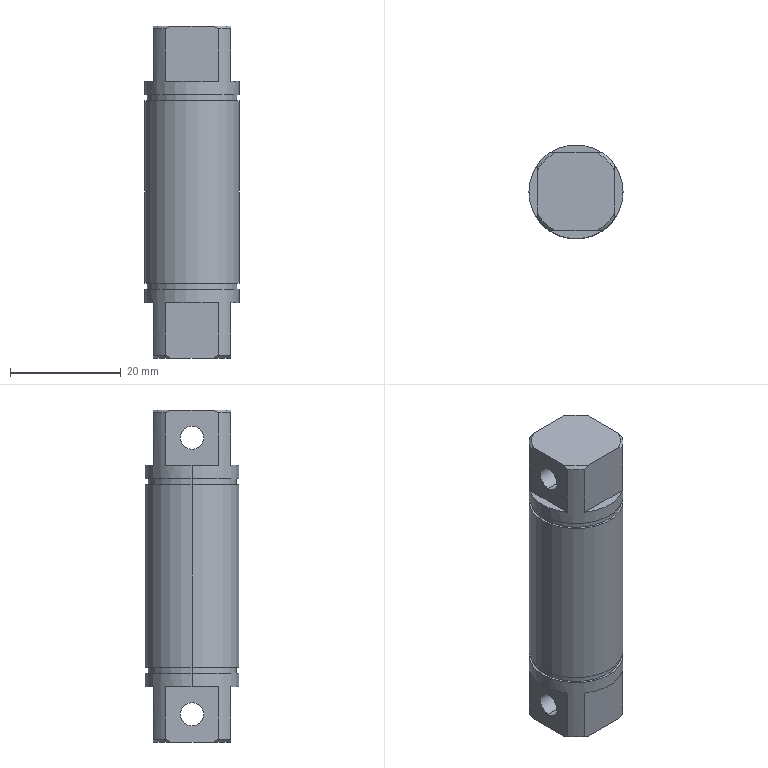Part | SolidWorks | features MirrorPattern 2, Chamfer 1, Extrusion 1, HoleWzd 1, ICE 1, RevCut 1 | 1 solid | 44 faces | box 17 x 17 x 60 mm | volume 12395 mm3 | plane 22 | cylinder 14 | cone 8 | commonest cylinder face diameters 17 x6 4.2 x4 16.2 x4
STEP:
#1=CARTESIAN_POINT('',(8.5,0.,20.));
#2=VERTEX_POINT('',#1);
#3=CARTESIAN_POINT('',(7.,4.822,20.));
#4=VERTEX_POINT('',#3);
#5=CARTESIAN_POINT('',(0.,0.,20.));
#6=DIRECTION('',(0.,0.,1.));
#7=DIRECTION('',(1.,0.,0.));
#8=AXIS2_PLACEMENT_3D('',#5,#6,#7);
#9=CIRCLE('',#8,8.5);
#10=EDGE_CURVE('',#2,#4,#9,.T.);
#11=ORIENTED_EDGE('',*,*,#10,.F.);
#12=CARTESIAN_POINT('',(8.5,0.,17.6));
#13=VERTEX_POINT('',#12);
#14=CARTESIAN_POINT('',(8.5,0.,30.));
#15=DIRECTION('',(0.,0.,-1.));
#16=VECTOR('',#15,1000.);
#17=LINE('',#14,#16);
#18=EDGE_CURVE('',#2,#13,#17,.T.);
#19=ORIENTED_EDGE('',*,*,#18,.T.);
#20=CARTESIAN_POINT('',(-8.5,0.,17.6));
#21=VERTEX_POINT('',#20);
#22=CARTESIAN_POINT('',(0.,0.,17.6));
#23=DIRECTION('',(0.,0.,-1.));
#24=DIRECTION('',(-1.,0.,0.));
#25=AXIS2_PLACEMENT_3D('',#22,#23,#24);
#26=CIRCLE('',#25,8.5);
#27=EDGE_CURVE('',#21,#13,#26,.T.);
#28=ORIENTED_EDGE('',*,*,#27,.F.);
#29=CARTESIAN_POINT('',(-8.5,0.,20.));
#30=VERTEX_POINT('',#29);
#31=CARTESIAN_POINT('',(-8.5,0.,30.));
#32=DIRECTION('',(0.,0.,-1.));
#33=VECTOR('',#32,1000.);
#34=LINE('',#31,#33);
#35=EDGE_CURVE('',#30,#21,#34,.T.);
#36=ORIENTED_EDGE('',*,*,#35,.F.);
#37=CARTESIAN_POINT('',(-7.,4.822,20.));
#38=VERTEX_POINT('',#37);
#39=CARTESIAN_POINT('',(0.,0.,20.));
#40=DIRECTION('',(0.,0.,1.));
#41=DIRECTION('',(1.,0.,0.));
#42=AXIS2_PLACEMENT_3D('',#39,#40,#41);
#43=CIRCLE('',#42,8.5);
#44=EDGE_CURVE('',#38,#30,#43,.T.);
#45=ORIENTED_EDGE('',*,*,#44,.F.);
#46=CARTESIAN_POINT('',(-7.,4.822,29.5));
#47=VERTEX_POINT('',#46);
#48=CARTESIAN_POINT('',(-7.,4.822,30.));
#49=DIRECTION('',(0.,0.,-1.));
#50=VECTOR('',#49,1000.);
#51=LINE('',#48,#50);
#52=EDGE_CURVE('',#47,#38,#51,.T.);
#53=ORIENTED_EDGE('',*,*,#52,.F.);
#54=CARTESIAN_POINT('',(-4.822,7.,29.5));
#55=VERTEX_POINT('',#54);
#56=CARTESIAN_POINT('',(0.,0.,29.5));
#57=DIRECTION('',(0.,0.,-1.));
#58=DIRECTION('',(1.,0.,0.));
#59=AXIS2_PLACEMENT_3D('',#56,#57,#58);
#60=CIRCLE('',#59,8.5);
#61=EDGE_CURVE('',#47,#55,#60,.T.);
#62=ORIENTED_EDGE('',*,*,#61,.T.);
#63=CARTESIAN_POINT('',(-4.822,7.,20.));
#64=VERTEX_POINT('',#63);
#65=CARTESIAN_POINT('',(-4.822,7.,30.));
#66=DIRECTION('',(0.,0.,1.));
#67=VECTOR('',#66,1000.);
#68=LINE('',#65,#67);
#69=EDGE_CURVE('',#64,#55,#68,.T.);
#70=ORIENTED_EDGE('',*,*,#69,.F.);
#71=CARTESIAN_POINT('',(4.822,7.,20.));
#72=VERTEX_POINT('',#71);
#73=CARTESIAN_POINT('',(0.,0.,20.));
#74=DIRECTION('',(0.,0.,1.));
#75=DIRECTION('',(1.,0.,0.));
#76=AXIS2_PLACEMENT_3D('',#73,#74,#75);
#77=CIRCLE('',#76,8.5);
#78=EDGE_CURVE('',#72,#64,#77,.T.);
#79=ORIENTED_EDGE('',*,*,#78,.F.);
#80=CARTESIAN_POINT('',(4.822,7.,29.5));
#81=VERTEX_POINT('',#80);
#82=CARTESIAN_POINT('',(4.822,7.,30.));
#83=DIRECTION('',(0.,0.,-1.));
#84=VECTOR('',#83,1000.);
#85=LINE('',#82,#84);
#86=EDGE_CURVE('',#81,#72,#85,.T.);
#87=ORIENTED_EDGE('',*,*,#86,.F.);
#88=CARTESIAN_POINT('',(7.,4.822,29.5));
#89=VERTEX_POINT('',#88);
#90=CARTESIAN_POINT('',(0.,0.,29.5));
#91=DIRECTION('',(0.,0.,-1.));
#92=DIRECTION('',(1.,0.,0.));
#93=AXIS2_PLACEMENT_3D('',#90,#91,#92);
#94=CIRCLE('',#93,8.5);
#95=EDGE_CURVE('',#81,#89,#94,.T.);
#96=ORIENTED_EDGE('',*,*,#95,.T.);
#97=CARTESIAN_POINT('',(7.,4.822,30.));
#98=DIRECTION('',(0.,0.,1.));
#99=VECTOR('',#98,1000.);
#100=LINE('',#97,#99);
#101=EDGE_CURVE('',#4,#89,#100,.T.);
#102=ORIENTED_EDGE('',*,*,#101,.F.);
#103=EDGE_LOOP('',(#11,#19,#28,#36,#45,#53,#62,#70,#79,#87,#96,#102));
#104=FACE_OUTER_BOUND('',#103,.T.);
#105=CARTESIAN_POINT('',(0.,0.,30.));
#106=DIRECTION('',(0.,0.,-1.));
#107=DIRECTION('',(-1.,0.,0.));
#108=AXIS2_PLACEMENT_3D('',#105,#106,#107);
#109=CYLINDRICAL_SURFACE('',#108,8.5);
#110=ADVANCED_FACE('',(#104),#109,.T.);
#111=CARTESIAN_POINT('',(-7.,0.,22.9));
#112=VERTEX_POINT('',#111);
#113=CARTESIAN_POINT('',(-7.,0.,27.1));
#114=VERTEX_POINT('',#113);
#115=CARTESIAN_POINT('',(-7.,0.,25.));
#116=DIRECTION('',(-1.,0.,0.));
#117=DIRECTION('',(0.,-1.,0.));
#118=AXIS2_PLACEMENT_3D('',#115,#116,#117);
#119=CIRCLE('',#118,2.1);
#120=EDGE_CURVE('',#112,#114,#119,.T.);
#121=ORIENTED_EDGE('',*,*,#120,.T.);
#122=CARTESIAN_POINT('',(7.,0.,27.1));
#123=VERTEX_POINT('',#122);
#124=CARTESIAN_POINT('',(7.,0.,27.1));
#125=DIRECTION('',(1.,0.,0.));
#126=VECTOR('',#125,1000.);
#127=LINE('',#124,#126);
#128=EDGE_CURVE('',#114,#123,#127,.T.);
#129=ORIENTED_EDGE('',*,*,#128,.T.);
#130=CARTESIAN_POINT('',(7.,0.,22.9));
#131=VERTEX_POINT('',#130);
#132=CARTESIAN_POINT('',(7.,0.,25.));
#133=DIRECTION('',(1.,0.,0.));
#134=DIRECTION('',(0.,0.,-1.));
#135=AXIS2_PLACEMENT_3D('',#132,#133,#134);
#136=CIRCLE('',#135,2.1);
#137=EDGE_CURVE('',#123,#131,#136,.T.);
#138=ORIENTED_EDGE('',*,*,#137,.T.);
#139=CARTESIAN_POINT('',(7.,0.,22.9));
#140=DIRECTION('',(1.,0.,0.));
#141=VECTOR('',#140,1000.);
#142=LINE('',#139,#141);
#143=EDGE_CURVE('',#112,#131,#142,.T.);
#144=ORIENTED_EDGE('',*,*,#143,.F.);
#145=EDGE_LOOP('',(#121,#129,#138,#144));
#146=FACE_OUTER_BOUND('',#145,.T.);
#147=CARTESIAN_POINT('',(7.,0.,25.));
#148=DIRECTION('',(1.,0.,0.));
#149=DIRECTION('',(0.,0.,-1.));
#150=AXIS2_PLACEMENT_3D('',#147,#148,#149);
#151=CYLINDRICAL_SURFACE('',#150,2.1);
#152=ADVANCED_FACE('',(#146),#151,.F.);
#153=CARTESIAN_POINT('',(8.1,0.,16.5));
#154=VERTEX_POINT('',#153);
#155=CARTESIAN_POINT('',(-8.1,0.,16.5));
#156=VERTEX_POINT('',#155);
#157=CARTESIAN_POINT('',(0.,0.,16.5));
#158=DIRECTION('',(0.,0.,-1.));
#159=DIRECTION('',(-1.,0.,0.));
#160=AXIS2_PLACEMENT_3D('',#157,#158,#159);
#161=CIRCLE('',#160,8.1);
#162=EDGE_CURVE('',#154,#156,#161,.T.);
#163=ORIENTED_EDGE('',*,*,#162,.F.);
#164=CARTESIAN_POINT('',(8.1,0.,17.6));
#165=VERTEX_POINT('',#164);
#166=CARTESIAN_POINT('',(8.1,0.,14.765));
#167=DIRECTION('',(0.,0.,1.));
#168=VECTOR('',#167,1000.);
#169=LINE('',#166,#168);
#170=EDGE_CURVE('',#154,#165,#169,.T.);
#171=ORIENTED_EDGE('',*,*,#170,.T.);
#172=CARTESIAN_POINT('',(-8.1,0.,17.6));
#173=VERTEX_POINT('',#172);
#174=CARTESIAN_POINT('',(0.,0.,17.6));
#175=DIRECTION('',(0.,0.,-1.));
#176=DIRECTION('',(-1.,0.,0.));
#177=AXIS2_PLACEMENT_3D('',#174,#175,#176);
#178=CIRCLE('',#177,8.1);
#179=EDGE_CURVE('',#165,#173,#178,.T.);
#180=ORIENTED_EDGE('',*,*,#179,.T.);
#181=CARTESIAN_POINT('',(-8.1,0.,14.765));
#182=DIRECTION('',(0.,0.,1.));
#183=VECTOR('',#182,1000.);
#184=LINE('',#181,#183);
#185=EDGE_CURVE('',#156,#173,#184,.T.);
#186=ORIENTED_EDGE('',*,*,#185,.F.);
#187=EDGE_LOOP('',(#163,#171,#180,#186));
#188=FACE_OUTER_BOUND('',#187,.T.);
#189=CARTESIAN_POINT('',(0.,0.,14.765));
#190=DIRECTION('',(0.,0.,1.));
#191=DIRECTION('',(-1.,0.,0.));
#192=AXIS2_PLACEMENT_3D('',#189,#190,#191);
#193=CYLINDRICAL_SURFACE('',#192,8.1);
#194=ADVANCED_FACE('',(#188),#193,.T.);
#195=CARTESIAN_POINT('',(-8.5,0.,-17.6));
#196=VERTEX_POINT('',#195);
#197=CARTESIAN_POINT('',(8.5,0.,-17.6));
#198=VERTEX_POINT('',#197);
#199=CARTESIAN_POINT('',(0.,0.,-17.6));
#200=DIRECTION('',(0.,0.,-1.));
#201=DIRECTION('',(-1.,0.,0.));
#202=AXIS2_PLACEMENT_3D('',#199,#200,#201);
#203=CIRCLE('',#202,8.5);
#204=EDGE_CURVE('',#196,#198,#203,.T.);
#205=ORIENTED_EDGE('',*,*,#204,.T.);
#206=CARTESIAN_POINT('',(8.5,0.,-20.));
#207=VERTEX_POINT('',#206);
#208=CARTESIAN_POINT('',(8.5,0.,30.));
#209=DIRECTION('',(0.,0.,-1.));
#210=VECTOR('',#209,1000.);
#211=LINE('',#208,#210);
#212=EDGE_CURVE('',#198,#207,#211,.T.);
#213=ORIENTED_EDGE('',*,*,#212,.T.);
#214=CARTESIAN_POINT('',(7.,4.822,-20.));
#215=VERTEX_POINT('',#214);
#216=CARTESIAN_POINT('',(0.,0.,-20.));
#217=DIRECTION('',(0.,0.,-1.));
#218=DIRECTION('',(-1.,0.,0.));
#219=AXIS2_PLACEMENT_3D('',#216,#217,#218);
#220=CIRCLE('',#219,8.5);
#221=EDGE_CURVE('',#215,#207,#220,.T.);
#222=ORIENTED_EDGE('',*,*,#221,.F.);
#223=CARTESIAN_POINT('',(7.,4.822,-29.5));
#224=VERTEX_POINT('',#223);
#225=CARTESIAN_POINT('',(7.,4.822,30.));
#226=DIRECTION('',(0.,0.,-1.));
#227=VECTOR('',#226,1000.);
#228=LINE('',#225,#227);
#229=EDGE_CURVE('',#215,#224,#228,.T.);
#230=ORIENTED_EDGE('',*,*,#229,.T.);
#231=CARTESIAN_POINT('',(4.822,7.,-29.5));
#232=VERTEX_POINT('',#231);
#233=CARTESIAN_POINT('',(0.,0.,-29.5));
#234=DIRECTION('',(0.,0.,1.));
#235=DIRECTION('',(1.,0.,0.));
#236=AXIS2_PLACEMENT_3D('',#233,#234,#235);
#237=CIRCLE('',#236,8.5);
#238=EDGE_CURVE('',#224,#232,#237,.T.);
#239=ORIENTED_EDGE('',*,*,#238,.T.);
#240=CARTESIAN_POINT('',(4.822,7.,-20.));
#241=VERTEX_POINT('',#240);
#242=CARTESIAN_POINT('',(4.822,7.,30.));
#243=DIRECTION('',(0.,0.,1.));
#244=VECTOR('',#243,1000.);
#245=LINE('',#242,#244);
#246=EDGE_CURVE('',#232,#241,#245,.T.);
#247=ORIENTED_EDGE('',*,*,#246,.T.);
#248=CARTESIAN_POINT('',(-4.822,7.,-20.));
#249=VERTEX_POINT('',#248);
#250=CARTESIAN_POINT('',(0.,0.,-20.));
#251=DIRECTION('',(0.,0.,-1.));
#252=DIRECTION('',(-1.,0.,0.));
#253=AXIS2_PLACEMENT_3D('',#250,#251,#252);
#254=CIRCLE('',#253,8.5);
#255=EDGE_CURVE('',#249,#241,#254,.T.);
#256=ORIENTED_EDGE('',*,*,#255,.F.);
#257=CARTESIAN_POINT('',(-4.822,7.,-29.5));
#258=VERTEX_POINT('',#257);
#259=CARTESIAN_POINT('',(-4.822,7.,30.));
#260=DIRECTION('',(0.,0.,-1.));
#261=VECTOR('',#260,1000.);
#262=LINE('',#259,#261);
#263=EDGE_CURVE('',#249,#258,#262,.T.);
#264=ORIENTED_EDGE('',*,*,#263,.T.);
#265=CARTESIAN_POINT('',(-7.,4.822,-29.5));
#266=VERTEX_POINT('',#265);
#267=CARTESIAN_POINT('',(0.,0.,-29.5));
#268=DIRECTION('',(0.,0.,1.));
#269=DIRECTION('',(1.,0.,0.));
#270=AXIS2_PLACEMENT_3D('',#267,#268,#269);
#271=CIRCLE('',#270,8.5);
#272=EDGE_CURVE('',#258,#266,#271,.T.);
#273=ORIENTED_EDGE('',*,*,#272,.T.);
#274=CARTESIAN_POINT('',(-7.,4.822,-20.));
#275=VERTEX_POINT('',#274);
#276=CARTESIAN_POINT('',(-7.,4.822,30.));
#277=DIRECTION('',(0.,0.,1.));
#278=VECTOR('',#277,1000.);
#279=LINE('',#276,#278);
#280=EDGE_CURVE('',#266,#275,#279,.T.);
#281=ORIENTED_EDGE('',*,*,#280,.T.);
#282=CARTESIAN_POINT('',(-8.5,0.,-20.));
#283=VERTEX_POINT('',#282);
#284=CARTESIAN_POINT('',(0.,0.,-20.));
#285=DIRECTION('',(0.,0.,-1.));
#286=DIRECTION('',(-1.,0.,0.));
#287=AXIS2_PLACEMENT_3D('',#284,#285,#286);
#288=CIRCLE('',#287,8.5);
#289=EDGE_CURVE('',#283,#275,#288,.T.);
#290=ORIENTED_EDGE('',*,*,#289,.F.);
#291=CARTESIAN_POINT('',(-8.5,0.,30.));
#292=DIRECTION('',(0.,0.,-1.));
#293=VECTOR('',#292,1000.);
#294=LINE('',#291,#293);
#295=EDGE_CURVE('',#196,#283,#294,.T.);
#296=ORIENTED_EDGE('',*,*,#295,.F.);
#297=EDGE_LOOP('',(#205,#213,#222,#230,#239,#247,#256,#264,#273,#281,#290,#296));
#298=FACE_OUTER_BOUND('',#297,.T.);
#299=CARTESIAN_POINT('',(0.,0.,30.));
#300=DIRECTION('',(0.,0.,-1.));
#301=DIRECTION('',(-1.,0.,0.));
#302=AXIS2_PLACEMENT_3D('',#299,#300,#301);
#303=CYLINDRICAL_SURFACE('',#302,8.5);
#304=ADVANCED_FACE('',(#298),#303,.T.);
#305=CARTESIAN_POINT('',(-7.,0.,-22.9));
#306=VERTEX_POINT('',#305);
#307=CARTESIAN_POINT('',(-7.,0.,-27.1));
#308=VERTEX_POINT('',#307);
#309=CARTESIAN_POINT('',(-7.,0.,-25.));
#310=DIRECTION('',(1.,0.,0.));
#311=DIRECTION('',(0.,1.,0.));
#312=AXIS2_PLACEMENT_3D('',#309,#310,#311);
#313=CIRCLE('',#312,2.1);
#314=EDGE_CURVE('',#306,#308,#313,.T.);
#315=ORIENTED_EDGE('',*,*,#314,.F.);
#316=CARTESIAN_POINT('',(7.,0.,-22.9));
#317=VERTEX_POINT('',#316);
#318=CARTESIAN_POINT('',(7.,0.,-22.9));
#319=DIRECTION('',(1.,0.,0.));
#320=VECTOR('',#319,1000.);
#321=LINE('',#318,#320);
#322=EDGE_CURVE('',#306,#317,#321,.T.);
#323=ORIENTED_EDGE('',*,*,#322,.T.);
#324=CARTESIAN_POINT('',(7.,0.,-27.1));
#325=VERTEX_POINT('',#324);
#326=CARTESIAN_POINT('',(7.,0.,-25.));
#327=DIRECTION('',(1.,0.,0.));
#328=DIRECTION('',(0.,0.,-1.));
#329=AXIS2_PLACEMENT_3D('',#326,#327,#328);
#330=CIRCLE('',#329,2.1);
#331=EDGE_CURVE('',#317,#325,#330,.T.);
#332=ORIENTED_EDGE('',*,*,#331,.T.);
#333=CARTESIAN_POINT('',(7.,0.,-27.1));
#334=DIRECTION('',(1.,0.,0.));
#335=VECTOR('',#334,1000.);
#336=LINE('',#333,#335);
#337=EDGE_CURVE('',#308,#325,#336,.T.);
#338=ORIENTED_EDGE('',*,*,#337,.F.);
#339=EDGE_LOOP('',(#315,#323,#332,#338));
#340=FACE_OUTER_BOUND('',#339,.T.);
#341=CARTESIAN_POINT('',(7.,0.,-25.));
#342=DIRECTION('',(1.,0.,0.));
#343=DIRECTION('',(0.,0.,-1.));
#344=AXIS2_PLACEMENT_3D('',#341,#342,#343);
#345=CYLINDRICAL_SURFACE('',#344,2.1);
#346=ADVANCED_FACE('',(#340),#345,.F.);
#347=CARTESIAN_POINT('',(-8.1,0.,-16.5));
#348=VERTEX_POINT('',#347);
#349=CARTESIAN_POINT('',(8.1,0.,-16.5));
#350=VERTEX_POINT('',#349);
#351=CARTESIAN_POINT('',(0.,0.,-16.5));
#352=DIRECTION('',(0.,0.,-1.));
#353=DIRECTION('',(-1.,0.,0.));
#354=AXIS2_PLACEMENT_3D('',#351,#352,#353);
#355=CIRCLE('',#354,8.1);
#356=EDGE_CURVE('',#348,#350,#355,.T.);
#357=ORIENTED_EDGE('',*,*,#356,.T.);
#358=CARTESIAN_POINT('',(8.1,0.,-17.6));
#359=VERTEX_POINT('',#358);
#360=CARTESIAN_POINT('',(8.1,0.,-14.765));
#361=DIRECTION('',(0.,0.,-1.));
#362=VECTOR('',#361,1000.);
#363=LINE('',#360,#362);
#364=EDGE_CURVE('',#350,#359,#363,.T.);
#365=ORIENTED_EDGE('',*,*,#364,.T.);
#366=CARTESIAN_POINT('',(-8.1,0.,-17.6));
#367=VERTEX_POINT('',#366);
#368=CARTESIAN_POINT('',(0.,0.,-17.6));
#369=DIRECTION('',(0.,0.,-1.));
#370=DIRECTION('',(-1.,0.,0.));
#371=AXIS2_PLACEMENT_3D('',#368,#369,#370);
#372=CIRCLE('',#371,8.1);
#373=EDGE_CURVE('',#367,#359,#372,.T.);
#374=ORIENTED_EDGE('',*,*,#373,.F.);
#375=CARTESIAN_POINT('',(-8.1,0.,-14.765));
#376=DIRECTION('',(0.,0.,-1.));
#377=VECTOR('',#376,1000.);
#378=LINE('',#375,#377);
#379=EDGE_CURVE('',#348,#367,#378,.T.);
#380=ORIENTED_EDGE('',*,*,#379,.F.);
#381=EDGE_LOOP('',(#357,#365,#374,#380));
#382=FACE_OUTER_BOUND('',#381,.T.);
#383=CARTESIAN_POINT('',(0.,0.,-14.765));
#384=DIRECTION('',(0.,0.,-1.));
#385=DIRECTION('',(-1.,0.,0.));
#386=AXIS2_PLACEMENT_3D('',#383,#384,#385);
#387=CYLINDRICAL_SURFACE('',#386,8.1);
#388=ADVANCED_FACE('',(#382),#387,.T.);
#389=CARTESIAN_POINT('',(-8.5,0.,16.5));
#390=VERTEX_POINT('',#389);
#391=CARTESIAN_POINT('',(8.5,0.,16.5));
#392=VERTEX_POINT('',#391);
#393=CARTESIAN_POINT('',(0.,0.,16.5));
#394=DIRECTION('',(0.,0.,-1.));
#395=DIRECTION('',(-1.,0.,0.));
#396=AXIS2_PLACEMENT_3D('',#393,#394,#395);
#397=CIRCLE('',#396,8.5);
#398=EDGE_CURVE('',#390,#392,#397,.T.);
#399=ORIENTED_EDGE('',*,*,#398,.T.);
#400=CARTESIAN_POINT('',(8.5,0.,-16.5));
#401=VERTEX_POINT('',#400);
#402=CARTESIAN_POINT('',(8.5,0.,30.));
#403=DIRECTION('',(0.,0.,-1.));
#404=VECTOR('',#403,1000.);
#405=LINE('',#402,#404);
#406=EDGE_CURVE('',#392,#401,#405,.T.);
#407=ORIENTED_EDGE('',*,*,#406,.T.);
#408=CARTESIAN_POINT('',(-8.5,0.,-16.5));
#409=VERTEX_POINT('',#408);
#410=CARTESIAN_POINT('',(0.,0.,-16.5));
#411=DIRECTION('',(0.,0.,-1.));
#412=DIRECTION('',(-1.,0.,0.));
#413=AXIS2_PLACEMENT_3D('',#410,#411,#412);
#414=CIRCLE('',#413,8.5);
#415=EDGE_CURVE('',#409,#401,#414,.T.);
#416=ORIENTED_EDGE('',*,*,#415,.F.);
#417=CARTESIAN_POINT('',(-8.5,0.,30.));
#418=DIRECTION('',(0.,0.,-1.));
#419=VECTOR('',#418,1000.);
#420=LINE('',#417,#419);
#421=EDGE_CURVE('',#390,#409,#420,.T.);
#422=ORIENTED_EDGE('',*,*,#421,.F.);
#423=EDGE_LOOP('',(#399,#407,#416,#422));
#424=FACE_OUTER_BOUND('',#423,.T.);
#425=CARTESIAN_POINT('',(0.,0.,30.));
#426=DIRECTION('',(0.,0.,-1.));
#427=DIRECTION('',(-1.,0.,0.));
#428=AXIS2_PLACEMENT_3D('',#425,#426,#427);
#429=CYLINDRICAL_SURFACE('',#428,8.5);
#430=ADVANCED_FACE('',(#424),#429,.T.);
#431=ORIENTED_EDGE('',*,*,#406,.F.);
#432=CARTESIAN_POINT('',(0.,0.,16.5));
#433=DIRECTION('',(0.,0.,-1.));
#434=DIRECTION('',(-1.,0.,0.));
#435=AXIS2_PLACEMENT_3D('',#432,#433,#434);
#436=CIRCLE('',#435,8.5);
#437=EDGE_CURVE('',#392,#390,#436,.T.);
#438=ORIENTED_EDGE('',*,*,#437,.T.);
#439=ORIENTED_EDGE('',*,*,#421,.T.);
#440=CARTESIAN_POINT('',(0.,0.,-16.5));
#441=DIRECTION('',(0.,0.,-1.));
#442=DIRECTION('',(-1.,0.,0.));
#443=AXIS2_PLACEMENT_3D('',#440,#441,#442);
#444=CIRCLE('',#443,8.5);
#445=EDGE_CURVE('',#401,#409,#444,.T.);
#446=ORIENTED_EDGE('',*,*,#445,.F.);
#447=EDGE_LOOP('',(#431,#438,#439,#446));
#448=FACE_OUTER_BOUND('',#447,.T.);
#449=CARTESIAN_POINT('',(0.,0.,30.));
#450=DIRECTION('',(0.,0.,-1.));
#451=DIRECTION('',(-1.,0.,0.));
#452=AXIS2_PLACEMENT_3D('',#449,#450,#451);
#453=CYLINDRICAL_SURFACE('',#452,8.5);
#454=ADVANCED_FACE('',(#448),#453,.T.);
#455=ORIENTED_EDGE('',*,*,#415,.T.);
#456=ORIENTED_EDGE('',*,*,#445,.T.);
#457=EDGE_LOOP('',(#455,#456));
#458=FACE_OUTER_BOUND('',#457,.T.);
#459=ORIENTED_EDGE('',*,*,#356,.F.);
#460=CARTESIAN_POINT('',(0.,0.,-16.5));
#461=DIRECTION('',(0.,0.,-1.));
#462=DIRECTION('',(-1.,0.,0.));
#463=AXIS2_PLACEMENT_3D('',#460,#461,#462);
#464=CIRCLE('',#463,8.1);
#465=EDGE_CURVE('',#350,#348,#464,.T.);
#466=ORIENTED_EDGE('',*,*,#465,.F.);
#467=EDGE_LOOP('',(#459,#466));
#468=FACE_BOUND('',#467,.T.);
#469=CARTESIAN_POINT('',(8.5,0.,-16.5));
#470=DIRECTION('',(0.,0.,-1.));
#471=DIRECTION('',(-1.,0.,0.));
#472=AXIS2_PLACEMENT_3D('',#469,#470,#471);
#473=PLANE('',#472);
#474=ADVANCED_FACE('',(#458,#468),#473,.T.);
#475=ORIENTED_EDGE('',*,*,#364,.F.);
#476=ORIENTED_EDGE('',*,*,#465,.T.);
#477=ORIENTED_EDGE('',*,*,#379,.T.);
#478=CARTESIAN_POINT('',(0.,0.,-17.6));
#479=DIRECTION('',(0.,0.,-1.));
#480=DIRECTION('',(-1.,0.,0.));
#481=AXIS2_PLACEMENT_3D('',#478,#479,#480);
#482=CIRCLE('',#481,8.1);
#483=EDGE_CURVE('',#359,#367,#482,.T.);
#484=ORIENTED_EDGE('',*,*,#483,.F.);
#485=EDGE_LOOP('',(#475,#476,#477,#484));
#486=FACE_OUTER_BOUND('',#485,.T.);
#487=CARTESIAN_POINT('',(0.,0.,-14.765));
#488=DIRECTION('',(0.,0.,-1.));
#489=DIRECTION('',(-1.,0.,0.));
#490=AXIS2_PLACEMENT_3D('',#487,#488,#489);
#491=CYLINDRICAL_SURFACE('',#490,8.1);
#492=ADVANCED_FACE('',(#486),#491,.T.);
#493=ORIENTED_EDGE('',*,*,#373,.T.);
#494=ORIENTED_EDGE('',*,*,#483,.T.);
#495=EDGE_LOOP('',(#493,#494));
#496=FACE_BOUND('',#495,.T.);
#497=ORIENTED_EDGE('',*,*,#204,.F.);
#498=CARTESIAN_POINT('',(0.,0.,-17.6));
#499=DIRECTION('',(0.,0.,-1.));
#500=DIRECTION('',(-1.,0.,0.));
#501=AXIS2_PLACEMENT_3D('',#498,#499,#500);
#502=CIRCLE('',#501,8.5);
#503=EDGE_CURVE('',#198,#196,#502,.T.);
#504=ORIENTED_EDGE('',*,*,#503,.F.);
#505=EDGE_LOOP('',(#497,#504));
#506=FACE_OUTER_BOUND('',#505,.T.);
#507=CARTESIAN_POINT('',(8.5,0.,-17.6));
#508=DIRECTION('',(0.,0.,1.));
#509=DIRECTION('',(1.,0.,0.));
#510=AXIS2_PLACEMENT_3D('',#507,#508,#509);
#511=PLANE('',#510);
#512=ADVANCED_FACE('',(#496,#506),#511,.T.);
#513=ORIENTED_EDGE('',*,*,#322,.F.);
#514=CARTESIAN_POINT('',(-7.,0.,-25.));
#515=DIRECTION('',(1.,0.,0.));
#516=DIRECTION('',(0.,1.,0.));
#517=AXIS2_PLACEMENT_3D('',#514,#515,#516);
#518=CIRCLE('',#517,2.1);
#519=EDGE_CURVE('',#308,#306,#518,.T.);
#520=ORIENTED_EDGE('',*,*,#519,.F.);
#521=ORIENTED_EDGE('',*,*,#337,.T.);
#522=CARTESIAN_POINT('',(7.,0.,-25.));
#523=DIRECTION('',(1.,0.,0.));
#524=DIRECTION('',(0.,0.,-1.));
#525=AXIS2_PLACEMENT_3D('',#522,#523,#524);
#526=CIRCLE('',#525,2.1);
#527=EDGE_CURVE('',#325,#317,#526,.T.);
#528=ORIENTED_EDGE('',*,*,#527,.T.);
#529=EDGE_LOOP('',(#513,#520,#521,#528));
#530=FACE_OUTER_BOUND('',#529,.T.);
#531=CARTESIAN_POINT('',(7.,0.,-25.));
#532=DIRECTION('',(1.,0.,0.));
#533=DIRECTION('',(0.,0.,-1.));
#534=AXIS2_PLACEMENT_3D('',#531,#532,#533);
#535=CYLINDRICAL_SURFACE('',#534,2.1);
#536=ADVANCED_FACE('',(#530),#535,.F.);
#537=CARTESIAN_POINT('',(7.,3.873,-30.));
#538=VERTEX_POINT('',#537);
#539=CARTESIAN_POINT('',(7.,-3.873,-30.));
#540=VERTEX_POINT('',#539);
#541=CARTESIAN_POINT('',(7.,0.,-30.));
#542=DIRECTION('',(0.,-1.,0.));
#543=VECTOR('',#542,1000.);
#544=LINE('',#541,#543);
#545=EDGE_CURVE('',#538,#540,#544,.T.);
#546=ORIENTED_EDGE('',*,*,#545,.T.);
#547=CARTESIAN_POINT('',(3.873,-7.,-30.));
#548=VERTEX_POINT('',#547);
#549=CARTESIAN_POINT('',(0.,0.,-30.));
#550=DIRECTION('',(0.,0.,-1.));
#551=DIRECTION('',(1.,0.,0.));
#552=AXIS2_PLACEMENT_3D('',#549,#550,#551);
#553=CIRCLE('',#552,8.);
#554=EDGE_CURVE('',#540,#548,#553,.T.);
#555=ORIENTED_EDGE('',*,*,#554,.T.);
#556=CARTESIAN_POINT('',(-3.873,-7.,-30.));
#557=VERTEX_POINT('',#556);
#558=CARTESIAN_POINT('',(0.,-7.,-30.));
#559=DIRECTION('',(-1.,0.,0.));
#560=VECTOR('',#559,1000.);
#561=LINE('',#558,#560);
#562=EDGE_CURVE('',#548,#557,#561,.T.);
#563=ORIENTED_EDGE('',*,*,#562,.T.);
#564=CARTESIAN_POINT('',(-7.,-3.873,-30.));
#565=VERTEX_POINT('',#564);
#566=CARTESIAN_POINT('',(0.,0.,-30.));
#567=DIRECTION('',(0.,0.,-1.));
#568=DIRECTION('',(1.,0.,0.));
#569=AXIS2_PLACEMENT_3D('',#566,#567,#568);
#570=CIRCLE('',#569,8.);
#571=EDGE_CURVE('',#557,#565,#570,.T.);
#572=ORIENTED_EDGE('',*,*,#571,.T.);
#573=CARTESIAN_POINT('',(-7.,3.873,-30.));
#574=VERTEX_POINT('',#573);
#575=CARTESIAN_POINT('',(-7.,0.,-30.));
#576=DIRECTION('',(0.,1.,0.));
#577=VECTOR('',#576,1000.);
#578=LINE('',#575,#577);
#579=EDGE_CURVE('',#565,#574,#578,.T.);
#580=ORIENTED_EDGE('',*,*,#579,.T.);
#581=CARTESIAN_POINT('',(-3.873,7.,-30.));
#582=VERTEX_POINT('',#581);
#583=CARTESIAN_POINT('',(0.,0.,-30.));
#584=DIRECTION('',(0.,0.,-1.));
#585=DIRECTION('',(1.,0.,0.));
#586=AXIS2_PLACEMENT_3D('',#583,#584,#585);
#587=CIRCLE('',#586,8.);
#588=EDGE_CURVE('',#574,#582,#587,.T.);
#589=ORIENTED_EDGE('',*,*,#588,.T.);
#590=CARTESIAN_POINT('',(3.873,7.,-30.));
#591=VERTEX_POINT('',#590);
#592=CARTESIAN_POINT('',(0.,7.,-30.));
#593=DIRECTION('',(1.,0.,0.));
#594=VECTOR('',#593,1000.);
#595=LINE('',#592,#594);
#596=EDGE_CURVE('',#582,#591,#595,.T.);
#597=ORIENTED_EDGE('',*,*,#596,.T.);
#598=CARTESIAN_POINT('',(0.,0.,-30.));
#599=DIRECTION('',(0.,0.,-1.));
#600=DIRECTION('',(1.,0.,0.));
#601=AXIS2_PLACEMENT_3D('',#598,#599,#600);
#602=CIRCLE('',#601,8.);
#603=EDGE_CURVE('',#591,#538,#602,.T.);
#604=ORIENTED_EDGE('',*,*,#603,.T.);
#605=EDGE_LOOP('',(#546,#555,#563,#572,#580,#589,#597,#604));
#606=FACE_OUTER_BOUND('',#605,.T.);
#607=CARTESIAN_POINT('',(0.,0.,-30.));
#608=DIRECTION('',(0.,0.,1.));
#609=DIRECTION('',(1.,0.,0.));
#610=AXIS2_PLACEMENT_3D('',#607,#608,#609);
#611=PLANE('',#610);
#612=ADVANCED_FACE('',(#606),#611,.F.);
#613=CARTESIAN_POINT('',(4.822,-7.,-20.));
#614=VERTEX_POINT('',#613);
#615=CARTESIAN_POINT('',(-4.822,-7.,-20.));
#616=VERTEX_POINT('',#615);
#617=CARTESIAN_POINT('',(0.,0.,-20.));
#618=DIRECTION('',(0.,0.,-1.));
#619=DIRECTION('',(-1.,0.,0.));
#620=AXIS2_PLACEMENT_3D('',#617,#618,#619);
#621=CIRCLE('',#620,8.5);
#622=EDGE_CURVE('',#614,#616,#621,.T.);
#623=ORIENTED_EDGE('',*,*,#622,.T.);
#624=CARTESIAN_POINT('',(-7.,-7.,-20.));
#625=DIRECTION('',(1.,0.,0.));
#626=VECTOR('',#625,1000.);
#627=LINE('',#624,#626);
#628=EDGE_CURVE('',#616,#614,#627,.T.);
#629=ORIENTED_EDGE('',*,*,#628,.T.);
#630=EDGE_LOOP('',(#623,#629));
#631=FACE_OUTER_BOUND('',#630,.T.);
#632=CARTESIAN_POINT('',(0.,0.,-20.));
#633=DIRECTION('',(0.,0.,-1.));
#634=DIRECTION('',(-1.,0.,0.));
#635=AXIS2_PLACEMENT_3D('',#632,#633,#634);
#636=PLANE('',#635);
#637=ADVANCED_FACE('',(#631),#636,.T.);
#638=CARTESIAN_POINT('',(-7.,-4.822,-29.5));
#639=VERTEX_POINT('',#638);
#640=CARTESIAN_POINT('',(-7.,-3.873,-30.));
#641=CARTESIAN_POINT('',(-7.,-4.195,-29.844));
#642=CARTESIAN_POINT('',(-7.,-4.511,-29.676));
#643=CARTESIAN_POINT('',(-7.,-4.822,-29.5));
#644=B_SPLINE_CURVE_WITH_KNOTS('',3,(#640,#641,#642,#643),.UNSPECIFIED.,.F.,.F.,(4,4),(0.,0.001073),.UNSPECIFIED.);
#645=EDGE_CURVE('',#565,#639,#644,.T.);
#646=ORIENTED_EDGE('',*,*,#645,.F.);
#647=ORIENTED_EDGE('',*,*,#571,.F.);
#648=CARTESIAN_POINT('',(-4.822,-7.,-29.5));
#649=VERTEX_POINT('',#648);
#650=CARTESIAN_POINT('',(-4.822,-7.,-29.5));
#651=CARTESIAN_POINT('',(-4.511,-7.,-29.676));
#652=CARTESIAN_POINT('',(-4.195,-7.,-29.844));
#653=CARTESIAN_POINT('',(-3.873,-7.,-30.));
#654=B_SPLINE_CURVE_WITH_KNOTS('',3,(#650,#651,#652,#653),.UNSPECIFIED.,.F.,.F.,(4,4),(0.,0.001073),.UNSPECIFIED.);
#655=EDGE_CURVE('',#649,#557,#654,.T.);
#656=ORIENTED_EDGE('',*,*,#655,.F.);
#657=CARTESIAN_POINT('',(0.,0.,-29.5));
#658=DIRECTION('',(0.,0.,1.));
#659=DIRECTION('',(1.,0.,0.));
#660=AXIS2_PLACEMENT_3D('',#657,#658,#659);
#661=CIRCLE('',#660,8.5);
#662=EDGE_CURVE('',#639,#649,#661,.T.);
#663=ORIENTED_EDGE('',*,*,#662,.F.);
#664=EDGE_LOOP('',(#646,#647,#656,#663));
#665=FACE_OUTER_BOUND('',#664,.T.);
#666=CARTESIAN_POINT('',(0.,0.,-29.5));
#667=DIRECTION('',(0.,0.,1.));
#668=DIRECTION('',(1.,0.,0.));
#669=AXIS2_PLACEMENT_3D('',#666,#667,#668);
#670=CONICAL_SURFACE('',#669,8.5,0.7854);
#671=ADVANCED_FACE('',(#665),#670,.T.);
#672=CARTESIAN_POINT('',(-7.,-4.822,-20.));
#673=VERTEX_POINT('',#672);
#674=CARTESIAN_POINT('',(0.,0.,-20.));
#675=DIRECTION('',(0.,0.,-1.));
#676=DIRECTION('',(-1.,0.,0.));
#677=AXIS2_PLACEMENT_3D('',#674,#675,#676);
#678=CIRCLE('',#677,8.5);
#679=EDGE_CURVE('',#673,#283,#678,.T.);
#680=ORIENTED_EDGE('',*,*,#679,.T.);
#681=ORIENTED_EDGE('',*,*,#289,.T.);
#682=CARTESIAN_POINT('',(-7.,7.,-20.));
#683=DIRECTION('',(0.,-1.,0.));
#684=VECTOR('',#683,1000.);
#685=LINE('',#682,#684);
#686=EDGE_CURVE('',#275,#673,#685,.T.);
#687=ORIENTED_EDGE('',*,*,#686,.T.);
#688=EDGE_LOOP('',(#680,#681,#687));
#689=FACE_OUTER_BOUND('',#688,.T.);
#690=CARTESIAN_POINT('',(0.,0.,-20.));
#691=DIRECTION('',(0.,0.,-1.));
#692=DIRECTION('',(-1.,0.,0.));
#693=AXIS2_PLACEMENT_3D('',#690,#691,#692);
#694=PLANE('',#693);
#695=ADVANCED_FACE('',(#689),#694,.T.);
#696=ORIENTED_EDGE('',*,*,#519,.T.);
#697=ORIENTED_EDGE('',*,*,#314,.T.);
#698=EDGE_LOOP('',(#696,#697));
#699=FACE_BOUND('',#698,.T.);
#700=ORIENTED_EDGE('',*,*,#280,.F.);
#701=CARTESIAN_POINT('',(-7.,4.822,-29.5));
#702=CARTESIAN_POINT('',(-7.,4.511,-29.676));
#703=CARTESIAN_POINT('',(-7.,4.195,-29.844));
#704=CARTESIAN_POINT('',(-7.,3.873,-30.));
#705=B_SPLINE_CURVE_WITH_KNOTS('',3,(#701,#702,#703,#704),.UNSPECIFIED.,.F.,.F.,(4,4),(0.,0.001073),.UNSPECIFIED.);
#706=EDGE_CURVE('',#266,#574,#705,.T.);
#707=ORIENTED_EDGE('',*,*,#706,.T.);
#708=ORIENTED_EDGE('',*,*,#579,.F.);
#709=ORIENTED_EDGE('',*,*,#645,.T.);
#710=CARTESIAN_POINT('',(-7.,-4.822,30.));
#711=DIRECTION('',(0.,0.,-1.));
#712=VECTOR('',#711,1000.);
#713=LINE('',#710,#712);
#714=EDGE_CURVE('',#673,#639,#713,.T.);
#715=ORIENTED_EDGE('',*,*,#714,.F.);
#716=ORIENTED_EDGE('',*,*,#686,.F.);
#717=EDGE_LOOP('',(#700,#707,#708,#709,#715,#716));
#718=FACE_OUTER_BOUND('',#717,.T.);
#719=CARTESIAN_POINT('',(-7.,7.,-20.));
#720=DIRECTION('',(1.,0.,0.));
#721=DIRECTION('',(0.,1.,0.));
#722=AXIS2_PLACEMENT_3D('',#719,#720,#721);
#723=PLANE('',#722);
#724=ADVANCED_FACE('',(#699,#718),#723,.F.);
#725=CARTESIAN_POINT('',(-3.873,7.,-30.));
#726=CARTESIAN_POINT('',(-4.195,7.,-29.844));
#727=CARTESIAN_POINT('',(-4.511,7.,-29.676));
#728=CARTESIAN_POINT('',(-4.822,7.,-29.5));
#729=B_SPLINE_CURVE_WITH_KNOTS('',3,(#725,#726,#727,#728),.UNSPECIFIED.,.F.,.F.,(4,4),(0.,0.001073),.UNSPECIFIED.);
#730=EDGE_CURVE('',#582,#258,#729,.T.);
#731=ORIENTED_EDGE('',*,*,#730,.F.);
#732=ORIENTED_EDGE('',*,*,#588,.F.);
#733=ORIENTED_EDGE('',*,*,#706,.F.);
#734=ORIENTED_EDGE('',*,*,#272,.F.);
#735=EDGE_LOOP('',(#731,#732,#733,#734));
#736=FACE_OUTER_BOUND('',#735,.T.);
#737=CARTESIAN_POINT('',(0.,0.,-29.5));
#738=DIRECTION('',(0.,0.,1.));
#739=DIRECTION('',(1.,0.,0.));
#740=AXIS2_PLACEMENT_3D('',#737,#738,#739);
#741=CONICAL_SURFACE('',#740,8.5,0.7854);
#742=ADVANCED_FACE('',(#736),#741,.T.);
#743=ORIENTED_EDGE('',*,*,#255,.T.);
#744=CARTESIAN_POINT('',(-7.,7.,-20.));
#745=DIRECTION('',(-1.,0.,0.));
#746=VECTOR('',#745,1000.);
#747=LINE('',#744,#746);
#748=EDGE_CURVE('',#241,#249,#747,.T.);
#749=ORIENTED_EDGE('',*,*,#748,.T.);
#750=EDGE_LOOP('',(#743,#749));
#751=FACE_OUTER_BOUND('',#750,.T.);
#752=CARTESIAN_POINT('',(0.,0.,-20.));
#753=DIRECTION('',(0.,0.,-1.));
#754=DIRECTION('',(-1.,0.,0.));
#755=AXIS2_PLACEMENT_3D('',#752,#753,#754);
#756=PLANE('',#755);
#757=ADVANCED_FACE('',(#751),#756,.T.);
#758=ORIENTED_EDGE('',*,*,#246,.F.);
#759=CARTESIAN_POINT('',(4.822,7.,-29.5));
#760=CARTESIAN_POINT('',(4.511,7.,-29.676));
#761=CARTESIAN_POINT('',(4.195,7.,-29.844));
#762=CARTESIAN_POINT('',(3.873,7.,-30.));
#763=B_SPLINE_CURVE_WITH_KNOTS('',3,(#759,#760,#761,#762),.UNSPECIFIED.,.F.,.F.,(4,4),(0.,0.001073),.UNSPECIFIED.);
#764=EDGE_CURVE('',#232,#591,#763,.T.);
#765=ORIENTED_EDGE('',*,*,#764,.T.);
#766=ORIENTED_EDGE('',*,*,#596,.F.);
#767=ORIENTED_EDGE('',*,*,#730,.T.);
#768=ORIENTED_EDGE('',*,*,#263,.F.);
#769=ORIENTED_EDGE('',*,*,#748,.F.);
#770=EDGE_LOOP('',(#758,#765,#766,#767,#768,#769));
#771=FACE_OUTER_BOUND('',#770,.T.);
#772=CARTESIAN_POINT('',(-7.,7.,-20.));
#773=DIRECTION('',(0.,-1.,0.));
#774=DIRECTION('',(0.,0.,-1.));
#775=AXIS2_PLACEMENT_3D('',#772,#773,#774);
#776=PLANE('',#775);
#777=ADVANCED_FACE('',(#771),#776,.F.);
#778=CARTESIAN_POINT('',(7.,3.873,-30.));
#779=CARTESIAN_POINT('',(7.,4.195,-29.844));
#780=CARTESIAN_POINT('',(7.,4.511,-29.676));
#781=CARTESIAN_POINT('',(7.,4.822,-29.5));
#782=B_SPLINE_CURVE_WITH_KNOTS('',3,(#778,#779,#780,#781),.UNSPECIFIED.,.F.,.F.,(4,4),(0.,0.001073),.UNSPECIFIED.);
#783=EDGE_CURVE('',#538,#224,#782,.T.);
#784=ORIENTED_EDGE('',*,*,#783,.F.);
#785=ORIENTED_EDGE('',*,*,#603,.F.);
#786=ORIENTED_EDGE('',*,*,#764,.F.);
#787=ORIENTED_EDGE('',*,*,#238,.F.);
#788=EDGE_LOOP('',(#784,#785,#786,#787));
#789=FACE_OUTER_BOUND('',#788,.T.);
#790=CARTESIAN_POINT('',(0.,0.,-29.5));
#791=DIRECTION('',(0.,0.,1.));
#792=DIRECTION('',(1.,0.,0.));
#793=AXIS2_PLACEMENT_3D('',#790,#791,#792);
#794=CONICAL_SURFACE('',#793,8.5,0.7854);
#795=ADVANCED_FACE('',(#789),#794,.T.);
#796=ORIENTED_EDGE('',*,*,#221,.T.);
#797=CARTESIAN_POINT('',(7.,-4.822,-20.));
#798=VERTEX_POINT('',#797);
#799=CARTESIAN_POINT('',(0.,0.,-20.));
#800=DIRECTION('',(0.,0.,-1.));
#801=DIRECTION('',(-1.,0.,0.));
#802=AXIS2_PLACEMENT_3D('',#799,#800,#801);
#803=CIRCLE('',#802,8.5);
#804=EDGE_CURVE('',#207,#798,#803,.T.);
#805=ORIENTED_EDGE('',*,*,#804,.T.);
#806=CARTESIAN_POINT('',(7.,7.,-20.));
#807=DIRECTION('',(0.,1.,0.));
#808=VECTOR('',#807,1000.);
#809=LINE('',#806,#808);
#810=EDGE_CURVE('',#798,#215,#809,.T.);
#811=ORIENTED_EDGE('',*,*,#810,.T.);
#812=EDGE_LOOP('',(#796,#805,#811));
#813=FACE_OUTER_BOUND('',#812,.T.);
#814=CARTESIAN_POINT('',(0.,0.,-20.));
#815=DIRECTION('',(0.,0.,-1.));
#816=DIRECTION('',(-1.,0.,0.));
#817=AXIS2_PLACEMENT_3D('',#814,#815,#816);
#818=PLANE('',#817);
#819=ADVANCED_FACE('',(#813),#818,.T.);
#820=CARTESIAN_POINT('',(7.,-4.822,-29.5));
#821=VERTEX_POINT('',#820);
#822=CARTESIAN_POINT('',(7.,-4.822,30.));
#823=DIRECTION('',(0.,0.,1.));
#824=VECTOR('',#823,1000.);
#825=LINE('',#822,#824);
#826=EDGE_CURVE('',#821,#798,#825,.T.);
#827=ORIENTED_EDGE('',*,*,#826,.F.);
#828=CARTESIAN_POINT('',(7.,-4.822,-29.5));
#829=CARTESIAN_POINT('',(7.,-4.511,-29.676));
#830=CARTESIAN_POINT('',(7.,-4.195,-29.844));
#831=CARTESIAN_POINT('',(7.,-3.873,-30.));
#832=B_SPLINE_CURVE_WITH_KNOTS('',3,(#828,#829,#830,#831),.UNSPECIFIED.,.F.,.F.,(4,4),(0.,0.001073),.UNSPECIFIED.);
#833=EDGE_CURVE('',#821,#540,#832,.T.);
#834=ORIENTED_EDGE('',*,*,#833,.T.);
#835=ORIENTED_EDGE('',*,*,#545,.F.);
#836=ORIENTED_EDGE('',*,*,#783,.T.);
#837=ORIENTED_EDGE('',*,*,#229,.F.);
#838=ORIENTED_EDGE('',*,*,#810,.F.);
#839=EDGE_LOOP('',(#827,#834,#835,#836,#837,#838));
#840=FACE_OUTER_BOUND('',#839,.T.);
#841=ORIENTED_EDGE('',*,*,#527,.F.);
#842=ORIENTED_EDGE('',*,*,#331,.F.);
#843=EDGE_LOOP('',(#841,#842));
#844=FACE_BOUND('',#843,.T.);
#845=CARTESIAN_POINT('',(7.,7.,-20.));
#846=DIRECTION('',(-1.,0.,0.));
#847=DIRECTION('',(0.,-1.,0.));
#848=AXIS2_PLACEMENT_3D('',#845,#846,#847);
#849=PLANE('',#848);
#850=ADVANCED_FACE('',(#840,#844),#849,.F.);
#851=CARTESIAN_POINT('',(4.822,-7.,-29.5));
#852=VERTEX_POINT('',#851);
#853=CARTESIAN_POINT('',(3.873,-7.,-30.));
#854=CARTESIAN_POINT('',(4.195,-7.,-29.844));
#855=CARTESIAN_POINT('',(4.511,-7.,-29.676));
#856=CARTESIAN_POINT('',(4.822,-7.,-29.5));
#857=B_SPLINE_CURVE_WITH_KNOTS('',3,(#853,#854,#855,#856),.UNSPECIFIED.,.F.,.F.,(4,4),(0.,0.001073),.UNSPECIFIED.);
#858=EDGE_CURVE('',#548,#852,#857,.T.);
#859=ORIENTED_EDGE('',*,*,#858,.F.);
#860=ORIENTED_EDGE('',*,*,#554,.F.);
#861=ORIENTED_EDGE('',*,*,#833,.F.);
#862=CARTESIAN_POINT('',(0.,0.,-29.5));
#863=DIRECTION('',(0.,0.,1.));
#864=DIRECTION('',(1.,0.,0.));
#865=AXIS2_PLACEMENT_3D('',#862,#863,#864);
#866=CIRCLE('',#865,8.5);
#867=EDGE_CURVE('',#852,#821,#866,.T.);
#868=ORIENTED_EDGE('',*,*,#867,.F.);
#869=EDGE_LOOP('',(#859,#860,#861,#868));
#870=FACE_OUTER_BOUND('',#869,.T.);
#871=CARTESIAN_POINT('',(0.,0.,-29.5));
#872=DIRECTION('',(0.,0.,1.));
#873=DIRECTION('',(1.,0.,0.));
#874=AXIS2_PLACEMENT_3D('',#871,#872,#873);
#875=CONICAL_SURFACE('',#874,8.5,0.7854);
#876=ADVANCED_FACE('',(#870),#875,.T.);
#877=ORIENTED_EDGE('',*,*,#562,.F.);
#878=ORIENTED_EDGE('',*,*,#858,.T.);
#879=CARTESIAN_POINT('',(4.822,-7.,30.));
#880=DIRECTION('',(0.,0.,-1.));
#881=VECTOR('',#880,1000.);
#882=LINE('',#879,#881);
#883=EDGE_CURVE('',#614,#852,#882,.T.);
#884=ORIENTED_EDGE('',*,*,#883,.F.);
#885=ORIENTED_EDGE('',*,*,#628,.F.);
#886=CARTESIAN_POINT('',(-4.822,-7.,30.));
#887=DIRECTION('',(0.,0.,1.));
#888=VECTOR('',#887,1000.);
#889=LINE('',#886,#888);
#890=EDGE_CURVE('',#649,#616,#889,.T.);
#891=ORIENTED_EDGE('',*,*,#890,.F.);
#892=ORIENTED_EDGE('',*,*,#655,.T.);
#893=EDGE_LOOP('',(#877,#878,#884,#885,#891,#892));
#894=FACE_OUTER_BOUND('',#893,.T.);
#895=CARTESIAN_POINT('',(-7.,-7.,-20.));
#896=DIRECTION('',(0.,1.,0.));
#897=DIRECTION('',(0.,0.,1.));
#898=AXIS2_PLACEMENT_3D('',#895,#896,#897);
#899=PLANE('',#898);
#900=ADVANCED_FACE('',(#894),#899,.F.);
#901=ORIENTED_EDGE('',*,*,#212,.F.);
#902=ORIENTED_EDGE('',*,*,#503,.T.);
#903=ORIENTED_EDGE('',*,*,#295,.T.);
#904=ORIENTED_EDGE('',*,*,#679,.F.);
#905=ORIENTED_EDGE('',*,*,#714,.T.);
#906=ORIENTED_EDGE('',*,*,#662,.T.);
#907=ORIENTED_EDGE('',*,*,#890,.T.);
#908=ORIENTED_EDGE('',*,*,#622,.F.);
#909=ORIENTED_EDGE('',*,*,#883,.T.);
#910=ORIENTED_EDGE('',*,*,#867,.T.);
#911=ORIENTED_EDGE('',*,*,#826,.T.);
#912=ORIENTED_EDGE('',*,*,#804,.F.);
#913=EDGE_LOOP('',(#901,#902,#903,#904,#905,#906,#907,#908,#909,#910,#911,#912));
#914=FACE_OUTER_BOUND('',#913,.T.);
#915=CARTESIAN_POINT('',(0.,0.,30.));
#916=DIRECTION('',(0.,0.,-1.));
#917=DIRECTION('',(-1.,0.,0.));
#918=AXIS2_PLACEMENT_3D('',#915,#916,#917);
#919=CYLINDRICAL_SURFACE('',#918,8.5);
#920=ADVANCED_FACE('',(#914),#919,.T.);
#921=ORIENTED_EDGE('',*,*,#398,.F.);
#922=ORIENTED_EDGE('',*,*,#437,.F.);
#923=EDGE_LOOP('',(#921,#922));
#924=FACE_OUTER_BOUND('',#923,.T.);
#925=CARTESIAN_POINT('',(0.,0.,16.5));
#926=DIRECTION('',(0.,0.,-1.));
#927=DIRECTION('',(-1.,0.,0.));
#928=AXIS2_PLACEMENT_3D('',#925,#926,#927);
#929=CIRCLE('',#928,8.1);
#930=EDGE_CURVE('',#156,#154,#929,.T.);
#931=ORIENTED_EDGE('',*,*,#930,.T.);
#932=ORIENTED_EDGE('',*,*,#162,.T.);
#933=EDGE_LOOP('',(#931,#932));
#934=FACE_BOUND('',#933,.T.);
#935=CARTESIAN_POINT('',(8.5,0.,16.5));
#936=DIRECTION('',(0.,0.,1.));
#937=DIRECTION('',(-1.,0.,0.));
#938=AXIS2_PLACEMENT_3D('',#935,#936,#937);
#939=PLANE('',#938);
#940=ADVANCED_FACE('',(#924,#934),#939,.T.);
#941=ORIENTED_EDGE('',*,*,#170,.F.);
#942=ORIENTED_EDGE('',*,*,#930,.F.);
#943=ORIENTED_EDGE('',*,*,#185,.T.);
#944=CARTESIAN_POINT('',(0.,0.,17.6));
#945=DIRECTION('',(0.,0.,-1.));
#946=DIRECTION('',(-1.,0.,0.));
#947=AXIS2_PLACEMENT_3D('',#944,#945,#946);
#948=CIRCLE('',#947,8.1);
#949=EDGE_CURVE('',#173,#165,#948,.T.);
#950=ORIENTED_EDGE('',*,*,#949,.T.);
#951=EDGE_LOOP('',(#941,#942,#943,#950));
#952=FACE_OUTER_BOUND('',#951,.T.);
#953=CARTESIAN_POINT('',(0.,0.,14.765));
#954=DIRECTION('',(0.,0.,1.));
#955=DIRECTION('',(-1.,0.,0.));
#956=AXIS2_PLACEMENT_3D('',#953,#954,#955);
#957=CYLINDRICAL_SURFACE('',#956,8.1);
#958=ADVANCED_FACE('',(#952),#957,.T.);
#959=ORIENTED_EDGE('',*,*,#949,.F.);
#960=ORIENTED_EDGE('',*,*,#179,.F.);
#961=EDGE_LOOP('',(#959,#960));
#962=FACE_BOUND('',#961,.T.);
#963=ORIENTED_EDGE('',*,*,#27,.T.);
#964=CARTESIAN_POINT('',(0.,0.,17.6));
#965=DIRECTION('',(0.,0.,-1.));
#966=DIRECTION('',(-1.,0.,0.));
#967=AXIS2_PLACEMENT_3D('',#964,#965,#966);
#968=CIRCLE('',#967,8.5);
#969=EDGE_CURVE('',#13,#21,#968,.T.);
#970=ORIENTED_EDGE('',*,*,#969,.T.);
#971=EDGE_LOOP('',(#963,#970));
#972=FACE_OUTER_BOUND('',#971,.T.);
#973=CARTESIAN_POINT('',(8.5,0.,17.6));
#974=DIRECTION('',(0.,0.,-1.));
#975=DIRECTION('',(1.,0.,0.));
#976=AXIS2_PLACEMENT_3D('',#973,#974,#975);
#977=PLANE('',#976);
#978=ADVANCED_FACE('',(#962,#972),#977,.T.);
#979=CARTESIAN_POINT('',(-3.873,-7.,30.));
#980=VERTEX_POINT('',#979);
#981=CARTESIAN_POINT('',(3.873,-7.,30.));
#982=VERTEX_POINT('',#981);
#983=CARTESIAN_POINT('',(0.,-7.,30.));
#984=DIRECTION('',(1.,0.,0.));
#985=VECTOR('',#984,1000.);
#986=LINE('',#983,#985);
#987=EDGE_CURVE('',#980,#982,#986,.T.);
#988=ORIENTED_EDGE('',*,*,#987,.T.);
#989=CARTESIAN_POINT('',(7.,-3.873,30.));
#990=VERTEX_POINT('',#989);
#991=CARTESIAN_POINT('',(0.,0.,30.));
#992=DIRECTION('',(0.,0.,1.));
#993=DIRECTION('',(1.,0.,0.));
#994=AXIS2_PLACEMENT_3D('',#991,#992,#993);
#995=CIRCLE('',#994,8.);
#996=EDGE_CURVE('',#982,#990,#995,.T.);
#997=ORIENTED_EDGE('',*,*,#996,.T.);
#998=CARTESIAN_POINT('',(7.,3.873,30.));
#999=VERTEX_POINT('',#998);
#1000=CARTESIAN_POINT('',(7.,0.,30.));
#1001=DIRECTION('',(0.,1.,0.));
#1002=VECTOR('',#1001,1000.);
#1003=LINE('',#1000,#1002);
#1004=EDGE_CURVE('',#990,#999,#1003,.T.);
#1005=ORIENTED_EDGE('',*,*,#1004,.T.);
#1006=CARTESIAN_POINT('',(3.873,7.,30.));
#1007=VERTEX_POINT('',#1006);
#1008=CARTESIAN_POINT('',(0.,0.,30.));
#1009=DIRECTION('',(0.,0.,1.));
#1010=DIRECTION('',(1.,0.,0.));
#1011=AXIS2_PLACEMENT_3D('',#1008,#1009,#1010);
#1012=CIRCLE('',#1011,8.);
#1013=EDGE_CURVE('',#999,#1007,#1012,.T.);
#1014=ORIENTED_EDGE('',*,*,#1013,.T.);
#1015=CARTESIAN_POINT('',(-3.873,7.,30.));
#1016=VERTEX_POINT('',#1015);
#1017=CARTESIAN_POINT('',(0.,7.,30.));
#1018=DIRECTION('',(-1.,0.,0.));
#1019=VECTOR('',#1018,1000.);
#1020=LINE('',#1017,#1019);
#1021=EDGE_CURVE('',#1007,#1016,#1020,.T.);
#1022=ORIENTED_EDGE('',*,*,#1021,.T.);
#1023=CARTESIAN_POINT('',(-7.,3.873,30.));
#1024=VERTEX_POINT('',#1023);
#1025=CARTESIAN_POINT('',(0.,0.,30.));
#1026=DIRECTION('',(0.,0.,1.));
#1027=DIRECTION('',(1.,0.,0.));
#1028=AXIS2_PLACEMENT_3D('',#1025,#1026,#1027);
#1029=CIRCLE('',#1028,8.);
#1030=EDGE_CURVE('',#1016,#1024,#1029,.T.);
#1031=ORIENTED_EDGE('',*,*,#1030,.T.);
#1032=CARTESIAN_POINT('',(-7.,-3.873,30.));
#1033=VERTEX_POINT('',#1032);
#1034=CARTESIAN_POINT('',(-7.,0.,30.));
#1035=DIRECTION('',(0.,-1.,0.));
#1036=VECTOR('',#1035,1000.);
#1037=LINE('',#1034,#1036);
#1038=EDGE_CURVE('',#1024,#1033,#1037,.T.);
#1039=ORIENTED_EDGE('',*,*,#1038,.T.);
#1040=CARTESIAN_POINT('',(0.,0.,30.));
#1041=DIRECTION('',(0.,0.,1.));
#1042=DIRECTION('',(1.,0.,0.));
#1043=AXIS2_PLACEMENT_3D('',#1040,#1041,#1042);
#1044=CIRCLE('',#1043,8.);
#1045=EDGE_CURVE('',#1033,#980,#1044,.T.);
#1046=ORIENTED_EDGE('',*,*,#1045,.T.);
#1047=EDGE_LOOP('',(#988,#997,#1005,#1014,#1022,#1031,#1039,#1046));
#1048=FACE_OUTER_BOUND('',#1047,.T.);
#1049=CARTESIAN_POINT('',(0.,0.,30.));
#1050=DIRECTION('',(0.,0.,1.));
#1051=DIRECTION('',(1.,0.,0.));
#1052=AXIS2_PLACEMENT_3D('',#1049,#1050,#1051);
#1053=PLANE('',#1052);
#1054=ADVANCED_FACE('',(#1048),#1053,.T.);
#1055=ORIENTED_EDGE('',*,*,#128,.F.);
#1056=CARTESIAN_POINT('',(-7.,0.,25.));
#1057=DIRECTION('',(-1.,0.,0.));
#1058=DIRECTION('',(0.,-1.,0.));
#1059=AXIS2_PLACEMENT_3D('',#1056,#1057,#1058);
#1060=CIRCLE('',#1059,2.1);
#1061=EDGE_CURVE('',#114,#112,#1060,.T.);
#1062=ORIENTED_EDGE('',*,*,#1061,.T.);
#1063=ORIENTED_EDGE('',*,*,#143,.T.);
#1064=CARTESIAN_POINT('',(7.,0.,25.));
#1065=DIRECTION('',(1.,0.,0.));
#1066=DIRECTION('',(0.,0.,-1.));
#1067=AXIS2_PLACEMENT_3D('',#1064,#1065,#1066);
#1068=CIRCLE('',#1067,2.1);
#1069=EDGE_CURVE('',#131,#123,#1068,.T.);
#1070=ORIENTED_EDGE('',*,*,#1069,.T.);
#1071=EDGE_LOOP('',(#1055,#1062,#1063,#1070));
#1072=FACE_OUTER_BOUND('',#1071,.T.);
#1073=CARTESIAN_POINT('',(7.,0.,25.));
#1074=DIRECTION('',(1.,0.,0.));
#1075=DIRECTION('',(0.,0.,-1.));
#1076=AXIS2_PLACEMENT_3D('',#1073,#1074,#1075);
#1077=CYLINDRICAL_SURFACE('',#1076,2.1);
#1078=ADVANCED_FACE('',(#1072),#1077,.F.);
#1079=CARTESIAN_POINT('',(7.,-4.822,20.));
#1080=VERTEX_POINT('',#1079);
#1081=CARTESIAN_POINT('',(0.,0.,20.));
#1082=DIRECTION('',(0.,0.,1.));
#1083=DIRECTION('',(1.,0.,0.));
#1084=AXIS2_PLACEMENT_3D('',#1081,#1082,#1083);
#1085=CIRCLE('',#1084,8.5);
#1086=EDGE_CURVE('',#1080,#2,#1085,.T.);
#1087=ORIENTED_EDGE('',*,*,#1086,.T.);
#1088=ORIENTED_EDGE('',*,*,#10,.T.);
#1089=CARTESIAN_POINT('',(7.,7.,20.));
#1090=DIRECTION('',(0.,1.,0.));
#1091=VECTOR('',#1090,1000.);
#1092=LINE('',#1089,#1091);
#1093=EDGE_CURVE('',#1080,#4,#1092,.T.);
#1094=ORIENTED_EDGE('',*,*,#1093,.F.);
#1095=EDGE_LOOP('',(#1087,#1088,#1094));
#1096=FACE_OUTER_BOUND('',#1095,.T.);
#1097=CARTESIAN_POINT('',(0.,0.,20.));
#1098=DIRECTION('',(0.,0.,1.));
#1099=DIRECTION('',(1.,0.,0.));
#1100=AXIS2_PLACEMENT_3D('',#1097,#1098,#1099);
#1101=PLANE('',#1100);
#1102=ADVANCED_FACE('',(#1096),#1101,.T.);
#1103=CARTESIAN_POINT('',(7.,4.822,29.5));
#1104=CARTESIAN_POINT('',(7.,4.511,29.676));
#1105=CARTESIAN_POINT('',(7.,4.195,29.844));
#1106=CARTESIAN_POINT('',(7.,3.873,30.));
#1107=B_SPLINE_CURVE_WITH_KNOTS('',3,(#1103,#1104,#1105,#1106),.UNSPECIFIED.,.F.,.F.,(4,4),(0.,0.001073),.UNSPECIFIED.);
#1108=EDGE_CURVE('',#89,#999,#1107,.T.);
#1109=ORIENTED_EDGE('',*,*,#1108,.F.);
#1110=ORIENTED_EDGE('',*,*,#95,.F.);
#1111=CARTESIAN_POINT('',(3.873,7.,30.));
#1112=CARTESIAN_POINT('',(4.195,7.,29.844));
#1113=CARTESIAN_POINT('',(4.511,7.,29.676));
#1114=CARTESIAN_POINT('',(4.822,7.,29.5));
#1115=B_SPLINE_CURVE_WITH_KNOTS('',3,(#1111,#1112,#1113,#1114),.UNSPECIFIED.,.F.,.F.,(4,4),(0.,0.001073),.UNSPECIFIED.);
#1116=EDGE_CURVE('',#1007,#81,#1115,.T.);
#1117=ORIENTED_EDGE('',*,*,#1116,.F.);
#1118=ORIENTED_EDGE('',*,*,#1013,.F.);
#1119=EDGE_LOOP('',(#1109,#1110,#1117,#1118));
#1120=FACE_OUTER_BOUND('',#1119,.T.);
#1121=CARTESIAN_POINT('',(0.,0.,30.));
#1122=DIRECTION('',(0.,0.,-1.));
#1123=DIRECTION('',(-1.,0.,0.));
#1124=AXIS2_PLACEMENT_3D('',#1121,#1122,#1123);
#1125=CONICAL_SURFACE('',#1124,8.,0.7854);
#1126=ADVANCED_FACE('',(#1120),#1125,.T.);
#1127=ORIENTED_EDGE('',*,*,#78,.T.);
#1128=CARTESIAN_POINT('',(-7.,7.,20.));
#1129=DIRECTION('',(-1.,0.,0.));
#1130=VECTOR('',#1129,1000.);
#1131=LINE('',#1128,#1130);
#1132=EDGE_CURVE('',#72,#64,#1131,.T.);
#1133=ORIENTED_EDGE('',*,*,#1132,.F.);
#1134=EDGE_LOOP('',(#1127,#1133));
#1135=FACE_OUTER_BOUND('',#1134,.T.);
#1136=CARTESIAN_POINT('',(0.,0.,20.));
#1137=DIRECTION('',(0.,0.,1.));
#1138=DIRECTION('',(1.,0.,0.));
#1139=AXIS2_PLACEMENT_3D('',#1136,#1137,#1138);
#1140=PLANE('',#1139);
#1141=ADVANCED_FACE('',(#1135),#1140,.T.);
#1142=ORIENTED_EDGE('',*,*,#69,.T.);
#1143=CARTESIAN_POINT('',(-4.822,7.,29.5));
#1144=CARTESIAN_POINT('',(-4.511,7.,29.676));
#1145=CARTESIAN_POINT('',(-4.195,7.,29.844));
#1146=CARTESIAN_POINT('',(-3.873,7.,30.));
#1147=B_SPLINE_CURVE_WITH_KNOTS('',3,(#1143,#1144,#1145,#1146),.UNSPECIFIED.,.F.,.F.,(4,4),(0.,0.001073),.UNSPECIFIED.);
#1148=EDGE_CURVE('',#55,#1016,#1147,.T.);
#1149=ORIENTED_EDGE('',*,*,#1148,.T.);
#1150=ORIENTED_EDGE('',*,*,#1021,.F.);
#1151=ORIENTED_EDGE('',*,*,#1116,.T.);
#1152=ORIENTED_EDGE('',*,*,#86,.T.);
#1153=ORIENTED_EDGE('',*,*,#1132,.T.);
#1154=EDGE_LOOP('',(#1142,#1149,#1150,#1151,#1152,#1153));
#1155=FACE_OUTER_BOUND('',#1154,.T.);
#1156=CARTESIAN_POINT('',(-7.,7.,20.));
#1157=DIRECTION('',(0.,1.,0.));
#1158=DIRECTION('',(0.,0.,1.));
#1159=AXIS2_PLACEMENT_3D('',#1156,#1157,#1158);
#1160=PLANE('',#1159);
#1161=ADVANCED_FACE('',(#1155),#1160,.T.);
#1162=ORIENTED_EDGE('',*,*,#1148,.F.);
#1163=ORIENTED_EDGE('',*,*,#61,.F.);
#1164=CARTESIAN_POINT('',(-7.,3.873,30.));
#1165=CARTESIAN_POINT('',(-7.,4.195,29.844));
#1166=CARTESIAN_POINT('',(-7.,4.511,29.676));
#1167=CARTESIAN_POINT('',(-7.,4.822,29.5));
#1168=B_SPLINE_CURVE_WITH_KNOTS('',3,(#1164,#1165,#1166,#1167),.UNSPECIFIED.,.F.,.F.,(4,4),(0.,0.001073),.UNSPECIFIED.);
#1169=EDGE_CURVE('',#1024,#47,#1168,.T.);
#1170=ORIENTED_EDGE('',*,*,#1169,.F.);
#1171=ORIENTED_EDGE('',*,*,#1030,.F.);
#1172=EDGE_LOOP('',(#1162,#1163,#1170,#1171));
#1173=FACE_OUTER_BOUND('',#1172,.T.);
#1174=CARTESIAN_POINT('',(0.,0.,30.));
#1175=DIRECTION('',(0.,0.,-1.));
#1176=DIRECTION('',(-1.,0.,0.));
#1177=AXIS2_PLACEMENT_3D('',#1174,#1175,#1176);
#1178=CONICAL_SURFACE('',#1177,8.,0.7854);
#1179=ADVANCED_FACE('',(#1173),#1178,.T.);
#1180=ORIENTED_EDGE('',*,*,#44,.T.);
#1181=CARTESIAN_POINT('',(-7.,-4.822,20.));
#1182=VERTEX_POINT('',#1181);
#1183=CARTESIAN_POINT('',(0.,0.,20.));
#1184=DIRECTION('',(0.,0.,1.));
#1185=DIRECTION('',(1.,0.,0.));
#1186=AXIS2_PLACEMENT_3D('',#1183,#1184,#1185);
#1187=CIRCLE('',#1186,8.5);
#1188=EDGE_CURVE('',#30,#1182,#1187,.T.);
#1189=ORIENTED_EDGE('',*,*,#1188,.T.);
#1190=CARTESIAN_POINT('',(-7.,7.,20.));
#1191=DIRECTION('',(0.,-1.,0.));
#1192=VECTOR('',#1191,1000.);
#1193=LINE('',#1190,#1192);
#1194=EDGE_CURVE('',#38,#1182,#1193,.T.);
#1195=ORIENTED_EDGE('',*,*,#1194,.F.);
#1196=EDGE_LOOP('',(#1180,#1189,#1195));
#1197=FACE_OUTER_BOUND('',#1196,.T.);
#1198=CARTESIAN_POINT('',(0.,0.,20.));
#1199=DIRECTION('',(0.,0.,1.));
#1200=DIRECTION('',(1.,0.,0.));
#1201=AXIS2_PLACEMENT_3D('',#1198,#1199,#1200);
#1202=PLANE('',#1201);
#1203=ADVANCED_FACE('',(#1197),#1202,.T.);
#1204=ORIENTED_EDGE('',*,*,#120,.F.);
#1205=ORIENTED_EDGE('',*,*,#1061,.F.);
#1206=EDGE_LOOP('',(#1204,#1205));
#1207=FACE_BOUND('',#1206,.T.);
#1208=CARTESIAN_POINT('',(-7.,-4.822,29.5));
#1209=VERTEX_POINT('',#1208);
#1210=CARTESIAN_POINT('',(-7.,-4.822,30.));
#1211=DIRECTION('',(0.,0.,1.));
#1212=VECTOR('',#1211,1000.);
#1213=LINE('',#1210,#1212);
#1214=EDGE_CURVE('',#1182,#1209,#1213,.T.);
#1215=ORIENTED_EDGE('',*,*,#1214,.T.);
#1216=CARTESIAN_POINT('',(-7.,-4.822,29.5));
#1217=CARTESIAN_POINT('',(-7.,-4.511,29.676));
#1218=CARTESIAN_POINT('',(-7.,-4.195,29.844));
#1219=CARTESIAN_POINT('',(-7.,-3.873,30.));
#1220=B_SPLINE_CURVE_WITH_KNOTS('',3,(#1216,#1217,#1218,#1219),.UNSPECIFIED.,.F.,.F.,(4,4),(0.,0.001073),.UNSPECIFIED.);
#1221=EDGE_CURVE('',#1209,#1033,#1220,.T.);
#1222=ORIENTED_EDGE('',*,*,#1221,.T.);
#1223=ORIENTED_EDGE('',*,*,#1038,.F.);
#1224=ORIENTED_EDGE('',*,*,#1169,.T.);
#1225=ORIENTED_EDGE('',*,*,#52,.T.);
#1226=ORIENTED_EDGE('',*,*,#1194,.T.);
#1227=EDGE_LOOP('',(#1215,#1222,#1223,#1224,#1225,#1226));
#1228=FACE_OUTER_BOUND('',#1227,.T.);
#1229=CARTESIAN_POINT('',(-7.,7.,20.));
#1230=DIRECTION('',(-1.,0.,0.));
#1231=DIRECTION('',(0.,-1.,0.));
#1232=AXIS2_PLACEMENT_3D('',#1229,#1230,#1231);
#1233=PLANE('',#1232);
#1234=ADVANCED_FACE('',(#1207,#1228),#1233,.T.);
#1235=ORIENTED_EDGE('',*,*,#1221,.F.);
#1236=CARTESIAN_POINT('',(-4.822,-7.,29.5));
#1237=VERTEX_POINT('',#1236);
#1238=CARTESIAN_POINT('',(0.,0.,29.5));
#1239=DIRECTION('',(0.,0.,-1.));
#1240=DIRECTION('',(1.,0.,0.));
#1241=AXIS2_PLACEMENT_3D('',#1238,#1239,#1240);
#1242=CIRCLE('',#1241,8.5);
#1243=EDGE_CURVE('',#1237,#1209,#1242,.T.);
#1244=ORIENTED_EDGE('',*,*,#1243,.F.);
#1245=CARTESIAN_POINT('',(-3.873,-7.,30.));
#1246=CARTESIAN_POINT('',(-4.195,-7.,29.844));
#1247=CARTESIAN_POINT('',(-4.511,-7.,29.676));
#1248=CARTESIAN_POINT('',(-4.822,-7.,29.5));
#1249=B_SPLINE_CURVE_WITH_KNOTS('',3,(#1245,#1246,#1247,#1248),.UNSPECIFIED.,.F.,.F.,(4,4),(0.,0.001073),.UNSPECIFIED.);
#1250=EDGE_CURVE('',#980,#1237,#1249,.T.);
#1251=ORIENTED_EDGE('',*,*,#1250,.F.);
#1252=ORIENTED_EDGE('',*,*,#1045,.F.);
#1253=EDGE_LOOP('',(#1235,#1244,#1251,#1252));
#1254=FACE_OUTER_BOUND('',#1253,.T.);
#1255=CARTESIAN_POINT('',(0.,0.,30.));
#1256=DIRECTION('',(0.,0.,-1.));
#1257=DIRECTION('',(-1.,0.,0.));
#1258=AXIS2_PLACEMENT_3D('',#1255,#1256,#1257);
#1259=CONICAL_SURFACE('',#1258,8.,0.7854);
#1260=ADVANCED_FACE('',(#1254),#1259,.T.);
#1261=CARTESIAN_POINT('',(-4.822,-7.,20.));
#1262=VERTEX_POINT('',#1261);
#1263=CARTESIAN_POINT('',(4.822,-7.,20.));
#1264=VERTEX_POINT('',#1263);
#1265=CARTESIAN_POINT('',(0.,0.,20.));
#1266=DIRECTION('',(0.,0.,1.));
#1267=DIRECTION('',(1.,0.,0.));
#1268=AXIS2_PLACEMENT_3D('',#1265,#1266,#1267);
#1269=CIRCLE('',#1268,8.5);
#1270=EDGE_CURVE('',#1262,#1264,#1269,.T.);
#1271=ORIENTED_EDGE('',*,*,#1270,.T.);
#1272=CARTESIAN_POINT('',(-7.,-7.,20.));
#1273=DIRECTION('',(1.,0.,0.));
#1274=VECTOR('',#1273,1000.);
#1275=LINE('',#1272,#1274);
#1276=EDGE_CURVE('',#1262,#1264,#1275,.T.);
#1277=ORIENTED_EDGE('',*,*,#1276,.F.);
#1278=EDGE_LOOP('',(#1271,#1277));
#1279=FACE_OUTER_BOUND('',#1278,.T.);
#1280=CARTESIAN_POINT('',(0.,0.,20.));
#1281=DIRECTION('',(0.,0.,1.));
#1282=DIRECTION('',(1.,0.,0.));
#1283=AXIS2_PLACEMENT_3D('',#1280,#1281,#1282);
#1284=PLANE('',#1283);
#1285=ADVANCED_FACE('',(#1279),#1284,.T.);
#1286=CARTESIAN_POINT('',(4.822,-7.,29.5));
#1287=VERTEX_POINT('',#1286);
#1288=CARTESIAN_POINT('',(4.822,-7.,30.));
#1289=DIRECTION('',(0.,0.,1.));
#1290=VECTOR('',#1289,1000.);
#1291=LINE('',#1288,#1290);
#1292=EDGE_CURVE('',#1264,#1287,#1291,.T.);
#1293=ORIENTED_EDGE('',*,*,#1292,.T.);
#1294=CARTESIAN_POINT('',(4.822,-7.,29.5));
#1295=CARTESIAN_POINT('',(4.511,-7.,29.676));
#1296=CARTESIAN_POINT('',(4.195,-7.,29.844));
#1297=CARTESIAN_POINT('',(3.873,-7.,30.));
#1298=B_SPLINE_CURVE_WITH_KNOTS('',3,(#1294,#1295,#1296,#1297),.UNSPECIFIED.,.F.,.F.,(4,4),(0.,0.001073),.UNSPECIFIED.);
#1299=EDGE_CURVE('',#1287,#982,#1298,.T.);
#1300=ORIENTED_EDGE('',*,*,#1299,.T.);
#1301=ORIENTED_EDGE('',*,*,#987,.F.);
#1302=ORIENTED_EDGE('',*,*,#1250,.T.);
#1303=CARTESIAN_POINT('',(-4.822,-7.,30.));
#1304=DIRECTION('',(0.,0.,-1.));
#1305=VECTOR('',#1304,1000.);
#1306=LINE('',#1303,#1305);
#1307=EDGE_CURVE('',#1237,#1262,#1306,.T.);
#1308=ORIENTED_EDGE('',*,*,#1307,.T.);
#1309=ORIENTED_EDGE('',*,*,#1276,.T.);
#1310=EDGE_LOOP('',(#1293,#1300,#1301,#1302,#1308,#1309));
#1311=FACE_OUTER_BOUND('',#1310,.T.);
#1312=CARTESIAN_POINT('',(-7.,-7.,20.));
#1313=DIRECTION('',(0.,-1.,0.));
#1314=DIRECTION('',(0.,0.,-1.));
#1315=AXIS2_PLACEMENT_3D('',#1312,#1313,#1314);
#1316=PLANE('',#1315);
#1317=ADVANCED_FACE('',(#1311),#1316,.T.);
#1318=ORIENTED_EDGE('',*,*,#1299,.F.);
#1319=CARTESIAN_POINT('',(7.,-4.822,29.5));
#1320=VERTEX_POINT('',#1319);
#1321=CARTESIAN_POINT('',(0.,0.,29.5));
#1322=DIRECTION('',(0.,0.,-1.));
#1323=DIRECTION('',(1.,0.,0.));
#1324=AXIS2_PLACEMENT_3D('',#1321,#1322,#1323);
#1325=CIRCLE('',#1324,8.5);
#1326=EDGE_CURVE('',#1320,#1287,#1325,.T.);
#1327=ORIENTED_EDGE('',*,*,#1326,.F.);
#1328=CARTESIAN_POINT('',(7.,-3.873,30.));
#1329=CARTESIAN_POINT('',(7.,-4.195,29.844));
#1330=CARTESIAN_POINT('',(7.,-4.511,29.676));
#1331=CARTESIAN_POINT('',(7.,-4.822,29.5));
#1332=B_SPLINE_CURVE_WITH_KNOTS('',3,(#1328,#1329,#1330,#1331),.UNSPECIFIED.,.F.,.F.,(4,4),(0.,0.001073),.UNSPECIFIED.);
#1333=EDGE_CURVE('',#990,#1320,#1332,.T.);
#1334=ORIENTED_EDGE('',*,*,#1333,.F.);
#1335=ORIENTED_EDGE('',*,*,#996,.F.);
#1336=EDGE_LOOP('',(#1318,#1327,#1334,#1335));
#1337=FACE_OUTER_BOUND('',#1336,.T.);
#1338=CARTESIAN_POINT('',(0.,0.,30.));
#1339=DIRECTION('',(0.,0.,-1.));
#1340=DIRECTION('',(-1.,0.,0.));
#1341=AXIS2_PLACEMENT_3D('',#1338,#1339,#1340);
#1342=CONICAL_SURFACE('',#1341,8.,0.7854);
#1343=ADVANCED_FACE('',(#1337),#1342,.T.);
#1344=ORIENTED_EDGE('',*,*,#1069,.F.);
#1345=ORIENTED_EDGE('',*,*,#137,.F.);
#1346=EDGE_LOOP('',(#1344,#1345));
#1347=FACE_BOUND('',#1346,.T.);
#1348=ORIENTED_EDGE('',*,*,#1004,.F.);
#1349=ORIENTED_EDGE('',*,*,#1333,.T.);
#1350=CARTESIAN_POINT('',(7.,-4.822,30.));
#1351=DIRECTION('',(0.,0.,-1.));
#1352=VECTOR('',#1351,1000.);
#1353=LINE('',#1350,#1352);
#1354=EDGE_CURVE('',#1320,#1080,#1353,.T.);
#1355=ORIENTED_EDGE('',*,*,#1354,.T.);
#1356=ORIENTED_EDGE('',*,*,#1093,.T.);
#1357=ORIENTED_EDGE('',*,*,#101,.T.);
#1358=ORIENTED_EDGE('',*,*,#1108,.T.);
#1359=EDGE_LOOP('',(#1348,#1349,#1355,#1356,#1357,#1358));
#1360=FACE_OUTER_BOUND('',#1359,.T.);
#1361=CARTESIAN_POINT('',(7.,7.,20.));
#1362=DIRECTION('',(1.,0.,0.));
#1363=DIRECTION('',(0.,1.,0.));
#1364=AXIS2_PLACEMENT_3D('',#1361,#1362,#1363);
#1365=PLANE('',#1364);
#1366=ADVANCED_FACE('',(#1347,#1360),#1365,.T.);
#1367=ORIENTED_EDGE('',*,*,#18,.F.);
#1368=ORIENTED_EDGE('',*,*,#1086,.F.);
#1369=ORIENTED_EDGE('',*,*,#1354,.F.);
#1370=ORIENTED_EDGE('',*,*,#1326,.T.);
#1371=ORIENTED_EDGE('',*,*,#1292,.F.);
#1372=ORIENTED_EDGE('',*,*,#1270,.F.);
#1373=ORIENTED_EDGE('',*,*,#1307,.F.);
#1374=ORIENTED_EDGE('',*,*,#1243,.T.);
#1375=ORIENTED_EDGE('',*,*,#1214,.F.);
#1376=ORIENTED_EDGE('',*,*,#1188,.F.);
#1377=ORIENTED_EDGE('',*,*,#35,.T.);
#1378=ORIENTED_EDGE('',*,*,#969,.F.);
#1379=EDGE_LOOP('',(#1367,#1368,#1369,#1370,#1371,#1372,#1373,#1374,#1375,#1376,#1377,#1378));
#1380=FACE_OUTER_BOUND('',#1379,.T.);
#1381=CARTESIAN_POINT('',(0.,0.,30.));
#1382=DIRECTION('',(0.,0.,-1.));
#1383=DIRECTION('',(-1.,0.,0.));
#1384=AXIS2_PLACEMENT_3D('',#1381,#1382,#1383);
#1385=CYLINDRICAL_SURFACE('',#1384,8.5);
#1386=ADVANCED_FACE('',(#1380),#1385,.T.);
#1387=CLOSED_SHELL('',(#110,#152,#194,#304,#346,#388,#430,#454,#474,#492,#512,#536,#612,#637,#671,#695,#724,#742,#757,#777,#795,#819,#850,#876,#900,#920,#940,#958,#978,#1054,#1078,#1102,#1126,#1141,#1161,#1179,#1203,#1234,#1260,#1285,#1317,#1343,#1366,#1386));
#1388=MANIFOLD_SOLID_BREP('',#1387);
#1389=CARTESIAN_POINT('',(0.,0.,0.));
#1390=DIRECTION('',(0.,0.,1.));
#1391=DIRECTION('',(1.,0.,0.));
#1392=AXIS2_PLACEMENT_3D('',#1389,#1390,#1391);
#1393=(LENGTH_UNIT()NAMED_UNIT(*)SI_UNIT(.MILLI.,.METRE.));
#1394=UNCERTAINTY_MEASURE_WITH_UNIT(LENGTH_MEASURE(0.00001),#1393,'','');
#1395=(NAMED_UNIT(*)PLANE_ANGLE_UNIT()SI_UNIT($,.RADIAN.));
#1396=(NAMED_UNIT(*)SI_UNIT($,.STERADIAN.)SOLID_ANGLE_UNIT());
#1397=(GEOMETRIC_REPRESENTATION_CONTEXT(3)GLOBAL_UNCERTAINTY_ASSIGNED_CONTEXT((#1394))GLOBAL_UNIT_ASSIGNED_CONTEXT((#1393,#1395,#1396))REPRESENTATION_CONTEXT('',''));
#1398=ADVANCED_BREP_SHAPE_REPRESENTATION('',(#1388,#1392),#1397);